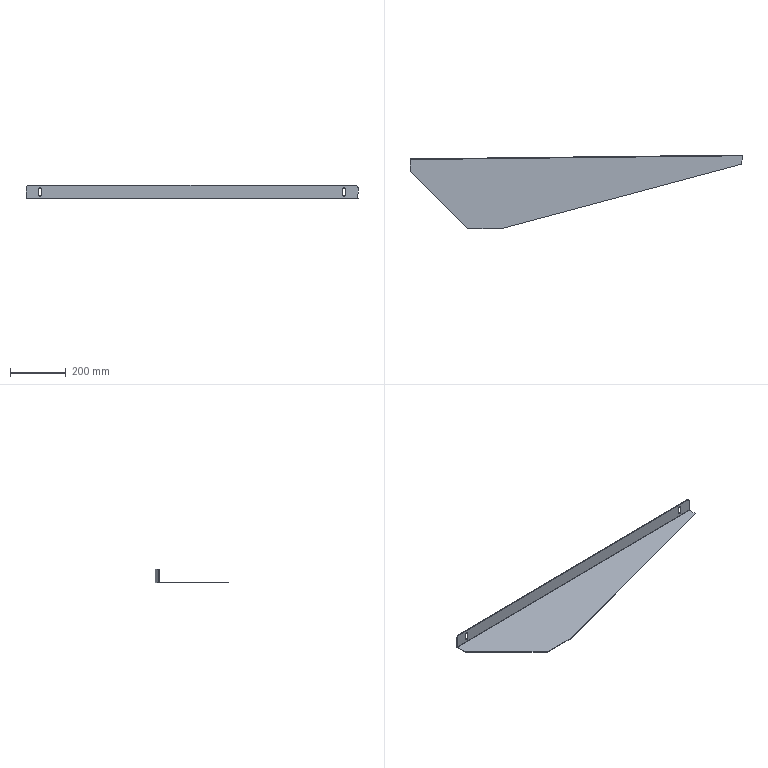Part | SolidWorks | features EdgeFlange 1, Extrusion 1, Fillet 1, FlatPattern 1, ICE 1, SheetMetal 1, SolidToSheetMetal 1 | 1 solid | 28 faces | box 1189 x 264.437 x 50 mm | volume 360864 mm3 | plane 19 | cylinder 8 | spline 1 | commonest cylinder face diameters 10 x4 20 x2 2 x1 5 x1
STEP:
#1=CARTESIAN_POINT('',(-18.814,-1.205,1.5));
#2=VERTEX_POINT('',#1);
#3=CARTESIAN_POINT('',(-18.814,-41.882,1.5));
#4=VERTEX_POINT('',#3);
#5=CARTESIAN_POINT('',(-18.814,0.5447,1.5));
#6=DIRECTION('',(0.,-1.,0.));
#7=VECTOR('',#6,1000.);
#8=LINE('',#5,#7);
#9=EDGE_CURVE('',#2,#4,#8,.T.);
#10=ORIENTED_EDGE('',*,*,#9,.F.);
#11=CARTESIAN_POINT('',(-18.814,-1.205,0.));
#12=VERTEX_POINT('',#11);
#13=CARTESIAN_POINT('',(-18.814,-1.205,1.5));
#14=DIRECTION('',(0.,0.,-1.));
#15=VECTOR('',#14,1000.);
#16=LINE('',#13,#15);
#17=EDGE_CURVE('',#2,#12,#16,.T.);
#18=ORIENTED_EDGE('',*,*,#17,.T.);
#19=CARTESIAN_POINT('',(-18.814,-41.882,0.));
#20=VERTEX_POINT('',#19);
#21=CARTESIAN_POINT('',(-18.814,0.,0.));
#22=DIRECTION('',(0.,-1.,0.));
#23=VECTOR('',#22,1000.);
#24=LINE('',#21,#23);
#25=EDGE_CURVE('',#12,#20,#24,.T.);
#26=ORIENTED_EDGE('',*,*,#25,.T.);
#27=CARTESIAN_POINT('',(-18.814,-41.882,1.5));
#28=DIRECTION('',(0.,0.,1.));
#29=VECTOR('',#28,1000.);
#30=LINE('',#27,#29);
#31=EDGE_CURVE('',#20,#4,#30,.T.);
#32=ORIENTED_EDGE('',*,*,#31,.T.);
#33=EDGE_LOOP('',(#10,#18,#26,#32));
#34=FACE_OUTER_BOUND('',#33,.T.);
#35=CARTESIAN_POINT('',(-18.814,0.5447,1.5));
#36=DIRECTION('',(-1.,0.,0.));
#37=DIRECTION('',(0.,-1.,0.));
#38=AXIS2_PLACEMENT_3D('',#35,#36,#37);
#39=PLANE('',#38);
#40=ADVANCED_FACE('',(#34),#39,.T.);
#41=CARTESIAN_POINT('',(-18.793,-1.205,1.5));
#42=VERTEX_POINT('',#41);
#43=CARTESIAN_POINT('',(-18.802,-0.4552,1.5));
#44=VERTEX_POINT('',#43);
#45=CARTESIAN_POINT('',(-18.793,-1.205,1.5));
#46=DIRECTION('',(-0.01155,0.9999,0.));
#47=VECTOR('',#46,1000.);
#48=LINE('',#45,#47);
#49=EDGE_CURVE('',#42,#44,#48,.T.);
#50=ORIENTED_EDGE('',*,*,#49,.F.);
#51=CARTESIAN_POINT('',(-19.543,-1.214,1.5));
#52=DIRECTION('',(0.9999,0.01155,0.));
#53=VECTOR('',#52,1000.);
#54=LINE('',#51,#53);
#55=EDGE_CURVE('',#2,#42,#54,.T.);
#56=ORIENTED_EDGE('',*,*,#55,.F.);
#57=ORIENTED_EDGE('',*,*,#9,.T.);
#58=CARTESIAN_POINT('',(187.963,-248.658,1.5));
#59=VERTEX_POINT('',#58);
#60=CARTESIAN_POINT('',(-18.814,-41.882,1.5));
#61=DIRECTION('',(0.7071,-0.7071,0.));
#62=VECTOR('',#61,1000.);
#63=LINE('',#60,#62);
#64=EDGE_CURVE('',#4,#59,#63,.T.);
#65=ORIENTED_EDGE('',*,*,#64,.T.);
#66=CARTESIAN_POINT('',(304.339,-248.658,1.5));
#67=VERTEX_POINT('',#66);
#68=CARTESIAN_POINT('',(187.963,-248.658,1.5));
#69=DIRECTION('',(1.,0.,0.));
#70=VECTOR('',#69,1000.);
#71=LINE('',#68,#70);
#72=EDGE_CURVE('',#59,#67,#71,.T.);
#73=ORIENTED_EDGE('',*,*,#72,.T.);
#74=CARTESIAN_POINT('',(1169.723,-16.78,1.5));
#75=VERTEX_POINT('',#74);
#76=CARTESIAN_POINT('',(304.339,-248.658,1.5));
#77=DIRECTION('',(0.9659,0.2588,0.));
#78=VECTOR('',#77,1000.);
#79=LINE('',#76,#78);
#80=EDGE_CURVE('',#67,#75,#79,.T.);
#81=ORIENTED_EDGE('',*,*,#80,.T.);
#82=CARTESIAN_POINT('',(1169.723,13.279,1.5));
#83=VERTEX_POINT('',#82);
#84=CARTESIAN_POINT('',(1169.723,14.279,1.5));
#85=DIRECTION('',(0.,1.,0.));
#86=VECTOR('',#85,1000.);
#87=LINE('',#84,#86);
#88=EDGE_CURVE('',#75,#83,#87,.T.);
#89=ORIENTED_EDGE('',*,*,#88,.T.);
#90=CARTESIAN_POINT('',(-18.802,-0.4552,1.5));
#91=DIRECTION('',(0.9999,0.01155,0.));
#92=VECTOR('',#91,1000.);
#93=LINE('',#90,#92);
#94=EDGE_CURVE('',#44,#83,#93,.T.);
#95=ORIENTED_EDGE('',*,*,#94,.F.);
#96=EDGE_LOOP('',(#50,#56,#57,#65,#73,#81,#89,#95));
#97=FACE_OUTER_BOUND('',#96,.T.);
#98=CARTESIAN_POINT('',(0.,0.,1.5));
#99=DIRECTION('',(0.,0.,1.));
#100=DIRECTION('',(1.,0.,0.));
#101=AXIS2_PLACEMENT_3D('',#98,#99,#100);
#102=PLANE('',#101);
#103=ADVANCED_FACE('',(#97),#102,.T.);
#104=CARTESIAN_POINT('',(-18.793,-1.205,0.));
#105=VERTEX_POINT('',#104);
#106=CARTESIAN_POINT('',(0.01141,-0.9878,0.));
#107=DIRECTION('',(-0.9999,-0.01155,0.));
#108=VECTOR('',#107,1000.);
#109=LINE('',#106,#108);
#110=EDGE_CURVE('',#105,#12,#109,.T.);
#111=ORIENTED_EDGE('',*,*,#110,.F.);
#112=CARTESIAN_POINT('',(-18.802,-0.4552,0.));
#113=VERTEX_POINT('',#112);
#114=CARTESIAN_POINT('',(-18.805,-0.2173,0.));
#115=DIRECTION('',(0.01155,-0.9999,0.));
#116=VECTOR('',#115,1000.);
#117=LINE('',#114,#116);
#118=EDGE_CURVE('',#113,#105,#117,.T.);
#119=ORIENTED_EDGE('',*,*,#118,.F.);
#120=CARTESIAN_POINT('',(1169.723,13.279,0.));
#121=VERTEX_POINT('',#120);
#122=CARTESIAN_POINT('',(-18.802,-0.4552,0.));
#123=DIRECTION('',(0.9999,0.01155,0.));
#124=VECTOR('',#123,1000.);
#125=LINE('',#122,#124);
#126=EDGE_CURVE('',#113,#121,#125,.T.);
#127=ORIENTED_EDGE('',*,*,#126,.T.);
#128=CARTESIAN_POINT('',(1169.723,-16.78,0.));
#129=VERTEX_POINT('',#128);
#130=CARTESIAN_POINT('',(1169.723,0.,0.));
#131=DIRECTION('',(0.,1.,0.));
#132=VECTOR('',#131,1000.);
#133=LINE('',#130,#132);
#134=EDGE_CURVE('',#129,#121,#133,.T.);
#135=ORIENTED_EDGE('',*,*,#134,.F.);
#136=CARTESIAN_POINT('',(304.339,-248.658,0.));
#137=VERTEX_POINT('',#136);
#138=CARTESIAN_POINT('',(304.339,-248.658,0.));
#139=DIRECTION('',(0.9659,0.2588,0.));
#140=VECTOR('',#139,1000.);
#141=LINE('',#138,#140);
#142=EDGE_CURVE('',#137,#129,#141,.T.);
#143=ORIENTED_EDGE('',*,*,#142,.F.);
#144=CARTESIAN_POINT('',(187.963,-248.658,0.));
#145=VERTEX_POINT('',#144);
#146=CARTESIAN_POINT('',(0.,-248.658,0.));
#147=DIRECTION('',(1.,0.,0.));
#148=VECTOR('',#147,1000.);
#149=LINE('',#146,#148);
#150=EDGE_CURVE('',#145,#137,#149,.T.);
#151=ORIENTED_EDGE('',*,*,#150,.F.);
#152=CARTESIAN_POINT('',(-18.814,-41.882,0.));
#153=DIRECTION('',(0.7071,-0.7071,0.));
#154=VECTOR('',#153,1000.);
#155=LINE('',#152,#154);
#156=EDGE_CURVE('',#20,#145,#155,.T.);
#157=ORIENTED_EDGE('',*,*,#156,.F.);
#158=ORIENTED_EDGE('',*,*,#25,.F.);
#159=EDGE_LOOP('',(#111,#119,#127,#135,#143,#151,#157,#158));
#160=FACE_OUTER_BOUND('',#159,.T.);
#161=CARTESIAN_POINT('',(0.,0.,0.));
#162=DIRECTION('',(0.,0.,1.));
#163=DIRECTION('',(1.,0.,0.));
#164=AXIS2_PLACEMENT_3D('',#161,#162,#163);
#165=PLANE('',#164);
#166=ADVANCED_FACE('',(#160),#165,.F.);
#167=ORIENTED_EDGE('',*,*,#31,.F.);
#168=ORIENTED_EDGE('',*,*,#156,.T.);
#169=CARTESIAN_POINT('',(187.963,-248.658,1.5));
#170=DIRECTION('',(0.,0.,1.));
#171=VECTOR('',#170,1000.);
#172=LINE('',#169,#171);
#173=EDGE_CURVE('',#145,#59,#172,.T.);
#174=ORIENTED_EDGE('',*,*,#173,.T.);
#175=ORIENTED_EDGE('',*,*,#64,.F.);
#176=EDGE_LOOP('',(#167,#168,#174,#175));
#177=FACE_OUTER_BOUND('',#176,.T.);
#178=CARTESIAN_POINT('',(-18.814,-41.882,1.5));
#179=DIRECTION('',(-0.7071,-0.7071,0.));
#180=DIRECTION('',(0.7071,-0.7071,0.));
#181=AXIS2_PLACEMENT_3D('',#178,#179,#180);
#182=PLANE('',#181);
#183=ADVANCED_FACE('',(#177),#182,.T.);
#184=ORIENTED_EDGE('',*,*,#173,.F.);
#185=ORIENTED_EDGE('',*,*,#150,.T.);
#186=CARTESIAN_POINT('',(304.339,-248.658,1.5));
#187=DIRECTION('',(0.,0.,1.));
#188=VECTOR('',#187,1000.);
#189=LINE('',#186,#188);
#190=EDGE_CURVE('',#137,#67,#189,.T.);
#191=ORIENTED_EDGE('',*,*,#190,.T.);
#192=ORIENTED_EDGE('',*,*,#72,.F.);
#193=EDGE_LOOP('',(#184,#185,#191,#192));
#194=FACE_OUTER_BOUND('',#193,.T.);
#195=CARTESIAN_POINT('',(187.963,-248.658,1.5));
#196=DIRECTION('',(0.,-1.,0.));
#197=DIRECTION('',(1.,0.,0.));
#198=AXIS2_PLACEMENT_3D('',#195,#196,#197);
#199=PLANE('',#198);
#200=ADVANCED_FACE('',(#194),#199,.T.);
#201=ORIENTED_EDGE('',*,*,#190,.F.);
#202=ORIENTED_EDGE('',*,*,#142,.T.);
#203=CARTESIAN_POINT('',(1169.723,-16.78,1.5));
#204=DIRECTION('',(0.,0.,1.));
#205=VECTOR('',#204,1000.);
#206=LINE('',#203,#205);
#207=EDGE_CURVE('',#129,#75,#206,.T.);
#208=ORIENTED_EDGE('',*,*,#207,.T.);
#209=ORIENTED_EDGE('',*,*,#80,.F.);
#210=EDGE_LOOP('',(#201,#202,#208,#209));
#211=FACE_OUTER_BOUND('',#210,.T.);
#212=CARTESIAN_POINT('',(304.339,-248.658,1.5));
#213=DIRECTION('',(0.2588,-0.9659,0.));
#214=DIRECTION('',(0.9659,0.2588,0.));
#215=AXIS2_PLACEMENT_3D('',#212,#213,#214);
#216=PLANE('',#215);
#217=ADVANCED_FACE('',(#211),#216,.T.);
#218=CARTESIAN_POINT('',(1169.723,13.279,1.5));
#219=DIRECTION('',(0.,0.,-1.));
#220=VECTOR('',#219,1000.);
#221=LINE('',#218,#220);
#222=EDGE_CURVE('',#83,#121,#221,.T.);
#223=ORIENTED_EDGE('',*,*,#222,.F.);
#224=ORIENTED_EDGE('',*,*,#88,.F.);
#225=ORIENTED_EDGE('',*,*,#207,.F.);
#226=ORIENTED_EDGE('',*,*,#134,.T.);
#227=EDGE_LOOP('',(#223,#224,#225,#226));
#228=FACE_OUTER_BOUND('',#227,.T.);
#229=CARTESIAN_POINT('',(1169.723,14.279,1.5));
#230=DIRECTION('',(1.,0.,0.));
#231=DIRECTION('',(0.,1.,0.));
#232=AXIS2_PLACEMENT_3D('',#229,#230,#231);
#233=PLANE('',#232);
#234=ADVANCED_FACE('',(#228),#233,.T.);
#235=CARTESIAN_POINT('',(-18.802,-0.4552,1.5));
#236=DIRECTION('',(0.,0.,-1.));
#237=VECTOR('',#236,1000.);
#238=LINE('',#235,#237);
#239=EDGE_CURVE('',#44,#113,#238,.T.);
#240=ORIENTED_EDGE('',*,*,#239,.T.);
#241=ORIENTED_EDGE('',*,*,#118,.T.);
#242=CARTESIAN_POINT('',(-18.793,-1.205,1.5));
#243=DIRECTION('',(0.,0.,-1.));
#244=VECTOR('',#243,1000.);
#245=LINE('',#242,#244);
#246=EDGE_CURVE('',#42,#105,#245,.T.);
#247=ORIENTED_EDGE('',*,*,#246,.F.);
#248=ORIENTED_EDGE('',*,*,#49,.T.);
#249=EDGE_LOOP('',(#240,#241,#247,#248));
#250=FACE_OUTER_BOUND('',#249,.T.);
#251=CARTESIAN_POINT('',(-18.793,-1.205,1.5));
#252=DIRECTION('',(-0.9999,-0.01155,0.));
#253=DIRECTION('',(0.01155,-0.9999,0.));
#254=AXIS2_PLACEMENT_3D('',#251,#252,#253);
#255=PLANE('',#254);
#256=ADVANCED_FACE('',(#250),#255,.T.);
#257=ORIENTED_EDGE('',*,*,#17,.F.);
#258=ORIENTED_EDGE('',*,*,#55,.T.);
#259=ORIENTED_EDGE('',*,*,#246,.T.);
#260=ORIENTED_EDGE('',*,*,#110,.T.);
#261=EDGE_LOOP('',(#257,#258,#259,#260));
#262=FACE_OUTER_BOUND('',#261,.T.);
#263=CARTESIAN_POINT('',(-19.543,-1.214,1.5));
#264=DIRECTION('',(-0.01155,0.9999,0.));
#265=DIRECTION('',(-0.9999,-0.01155,0.));
#266=AXIS2_PLACEMENT_3D('',#263,#264,#265);
#267=PLANE('',#266);
#268=ADVANCED_FACE('',(#262),#267,.T.);
#269=CARTESIAN_POINT('',(1169.723,14.279,2.5));
#270=VERTEX_POINT('',#269);
#271=CARTESIAN_POINT('',(1169.705,15.779,2.5));
#272=VERTEX_POINT('',#271);
#273=CARTESIAN_POINT('',(1169.723,14.279,2.5));
#274=DIRECTION('',(-0.01155,0.9999,0.));
#275=VECTOR('',#274,1000.);
#276=LINE('',#273,#275);
#277=EDGE_CURVE('',#270,#272,#276,.T.);
#278=ORIENTED_EDGE('',*,*,#277,.F.);
#279=CARTESIAN_POINT('',(1169.723,13.279,1.5));
#280=CARTESIAN_POINT('',(1169.722,13.541,1.5));
#281=CARTESIAN_POINT('',(1169.721,13.801,1.608));
#282=CARTESIAN_POINT('',(1169.72,14.171,1.978));
#283=CARTESIAN_POINT('',(1169.721,14.279,2.238));
#284=CARTESIAN_POINT('',(1169.723,14.279,2.5));
#285=B_SPLINE_CURVE_WITH_KNOTS('',3,(#279,#280,#281,#282,#283,#284),.UNSPECIFIED.,.F.,.F.,(4,2,4),(0.,0.5,1.),.UNSPECIFIED.);
#286=EDGE_CURVE('',#83,#270,#285,.T.);
#287=ORIENTED_EDGE('',*,*,#286,.F.);
#288=ORIENTED_EDGE('',*,*,#222,.T.);
#289=CARTESIAN_POINT('',(1169.723,13.279,0.));
#290=CARTESIAN_POINT('',(1169.72,13.606,0.));
#291=CARTESIAN_POINT('',(1169.717,13.933,0.06507));
#292=CARTESIAN_POINT('',(1169.712,14.538,0.3155));
#293=CARTESIAN_POINT('',(1169.71,14.815,0.5008));
#294=CARTESIAN_POINT('',(1169.706,15.278,0.9636));
#295=CARTESIAN_POINT('',(1169.705,15.463,1.241));
#296=CARTESIAN_POINT('',(1169.704,15.714,1.846));
#297=CARTESIAN_POINT('',(1169.704,15.779,2.173));
#298=CARTESIAN_POINT('',(1169.705,15.779,2.5));
#299=B_SPLINE_CURVE_WITH_KNOTS('',3,(#289,#290,#291,#292,#293,#294,#295,#296,#297,#298),.UNSPECIFIED.,.F.,.F.,(4,2,2,2,4),(0.,0.25,0.5,0.75,1.),.UNSPECIFIED.);
#300=EDGE_CURVE('',#121,#272,#299,.T.);
#301=ORIENTED_EDGE('',*,*,#300,.T.);
#302=EDGE_LOOP('',(#278,#287,#288,#301));
#303=FACE_OUTER_BOUND('',#302,.T.);
#304=CARTESIAN_POINT('',(1169.723,13.279,-0.015));
#305=CARTESIAN_POINT('',(1169.72,13.608,-0.015));
#306=CARTESIAN_POINT('',(1169.717,13.937,0.05046));
#307=CARTESIAN_POINT('',(1169.712,14.545,0.3024));
#308=CARTESIAN_POINT('',(1169.71,14.824,0.4888));
#309=CARTESIAN_POINT('',(1169.706,15.29,0.9544));
#310=CARTESIAN_POINT('',(1169.705,15.476,1.233));
#311=CARTESIAN_POINT('',(1169.704,15.728,1.842));
#312=CARTESIAN_POINT('',(1169.704,15.794,2.171));
#313=CARTESIAN_POINT('',(1169.705,15.794,2.5));
#314=CARTESIAN_POINT('',(1169.723,13.279,0.));
#315=CARTESIAN_POINT('',(1169.72,13.606,0.));
#316=CARTESIAN_POINT('',(1169.717,13.933,0.06507));
#317=CARTESIAN_POINT('',(1169.712,14.538,0.3155));
#318=CARTESIAN_POINT('',(1169.71,14.815,0.5008));
#319=CARTESIAN_POINT('',(1169.706,15.278,0.9636));
#320=CARTESIAN_POINT('',(1169.705,15.463,1.241));
#321=CARTESIAN_POINT('',(1169.704,15.714,1.846));
#322=CARTESIAN_POINT('',(1169.704,15.779,2.173));
#323=CARTESIAN_POINT('',(1169.705,15.779,2.5));
#324=CARTESIAN_POINT('',(1169.723,13.279,1.5));
#325=CARTESIAN_POINT('',(1169.722,13.41,1.5));
#326=CARTESIAN_POINT('',(1169.722,13.54,1.526));
#327=CARTESIAN_POINT('',(1169.721,13.782,1.626));
#328=CARTESIAN_POINT('',(1169.72,13.893,1.7));
#329=CARTESIAN_POINT('',(1169.72,14.078,1.885));
#330=CARTESIAN_POINT('',(1169.72,14.153,1.996));
#331=CARTESIAN_POINT('',(1169.721,14.253,2.238));
#332=CARTESIAN_POINT('',(1169.722,14.279,2.369));
#333=CARTESIAN_POINT('',(1169.723,14.279,2.5));
#334=CARTESIAN_POINT('',(1169.723,13.279,1.515));
#335=CARTESIAN_POINT('',(1169.722,13.408,1.515));
#336=CARTESIAN_POINT('',(1169.722,13.537,1.541));
#337=CARTESIAN_POINT('',(1169.721,13.775,1.639));
#338=CARTESIAN_POINT('',(1169.721,13.884,1.712));
#339=CARTESIAN_POINT('',(1169.72,14.066,1.895));
#340=CARTESIAN_POINT('',(1169.72,14.139,2.004));
#341=CARTESIAN_POINT('',(1169.721,14.238,2.242));
#342=CARTESIAN_POINT('',(1169.722,14.264,2.371));
#343=CARTESIAN_POINT('',(1169.723,14.264,2.5));
#344=B_SPLINE_SURFACE_WITH_KNOTS('',1,3,((#304,#305,#306,#307,#308,#309,#310,#311,#312,#313),(#314,#315,#316,#317,#318,#319,#320,#321,#322,#323),(#324,#325,#326,#327,#328,#329,#330,#331,#332,#333),(#334,#335,#336,#337,#338,#339,#340,#341,#342,#343)),.UNSPECIFIED.,.F.,.F.,.F.,(2,1,1,2),(4,2,2,2,4),(-0.01,0.,1.,1.01),(0.,0.25,0.5,0.75,1.),.UNSPECIFIED.);
#345=ADVANCED_FACE('',(#303),#344,.F.);
#346=CARTESIAN_POINT('',(-18.814,0.5447,2.5));
#347=VERTEX_POINT('',#346);
#348=CARTESIAN_POINT('',(-18.802,-0.4552,2.5));
#349=DIRECTION('',(-0.9999,-0.01155,0.));
#350=DIRECTION('',(0.01155,-0.9999,0.));
#351=AXIS2_PLACEMENT_3D('',#348,#349,#350);
#352=CIRCLE('',#351,1.);
#353=EDGE_CURVE('',#347,#44,#352,.T.);
#354=ORIENTED_EDGE('',*,*,#353,.F.);
#355=CARTESIAN_POINT('',(-18.831,2.045,2.5));
#356=VERTEX_POINT('',#355);
#357=CARTESIAN_POINT('',(-18.814,0.5447,2.5));
#358=DIRECTION('',(-0.01155,0.9999,0.));
#359=VECTOR('',#358,1000.);
#360=LINE('',#357,#359);
#361=EDGE_CURVE('',#347,#356,#360,.T.);
#362=ORIENTED_EDGE('',*,*,#361,.T.);
#363=CARTESIAN_POINT('',(-18.802,-0.4552,2.5));
#364=DIRECTION('',(-0.9999,-0.01155,0.));
#365=DIRECTION('',(0.01155,-0.9999,0.));
#366=AXIS2_PLACEMENT_3D('',#363,#364,#365);
#367=CIRCLE('',#366,2.5);
#368=EDGE_CURVE('',#356,#113,#367,.T.);
#369=ORIENTED_EDGE('',*,*,#368,.T.);
#370=ORIENTED_EDGE('',*,*,#239,.F.);
#371=EDGE_LOOP('',(#354,#362,#369,#370));
#372=FACE_OUTER_BOUND('',#371,.T.);
#373=CARTESIAN_POINT('',(-18.802,-0.4552,2.5));
#374=DIRECTION('',(0.9999,0.01155,0.));
#375=DIRECTION('',(-0.01155,0.9999,0.));
#376=AXIS2_PLACEMENT_3D('',#373,#374,#375);
#377=PLANE('',#376);
#378=ADVANCED_FACE('',(#372),#377,.F.);
#379=ORIENTED_EDGE('',*,*,#126,.F.);
#380=ORIENTED_EDGE('',*,*,#368,.F.);
#381=CARTESIAN_POINT('',(-0.02614,2.262,2.5));
#382=DIRECTION('',(0.9999,0.01155,0.));
#383=VECTOR('',#382,1000.);
#384=LINE('',#381,#383);
#385=EDGE_CURVE('',#356,#272,#384,.T.);
#386=ORIENTED_EDGE('',*,*,#385,.T.);
#387=ORIENTED_EDGE('',*,*,#300,.F.);
#388=EDGE_LOOP('',(#379,#380,#386,#387));
#389=FACE_OUTER_BOUND('',#388,.T.);
#390=CARTESIAN_POINT('',(-18.802,-0.4552,2.5));
#391=DIRECTION('',(-0.9999,-0.01155,0.));
#392=DIRECTION('',(-0.01155,0.9999,0.));
#393=AXIS2_PLACEMENT_3D('',#390,#391,#392);
#394=CYLINDRICAL_SURFACE('',#393,2.5);
#395=ADVANCED_FACE('',(#389),#394,.T.);
#396=ORIENTED_EDGE('',*,*,#94,.T.);
#397=ORIENTED_EDGE('',*,*,#286,.T.);
#398=CARTESIAN_POINT('',(1169.723,14.279,2.5));
#399=DIRECTION('',(-0.9999,-0.01155,0.));
#400=VECTOR('',#399,1000.);
#401=LINE('',#398,#400);
#402=EDGE_CURVE('',#270,#347,#401,.T.);
#403=ORIENTED_EDGE('',*,*,#402,.T.);
#404=ORIENTED_EDGE('',*,*,#353,.T.);
#405=EDGE_LOOP('',(#396,#397,#403,#404));
#406=FACE_OUTER_BOUND('',#405,.T.);
#407=CARTESIAN_POINT('',(-18.802,-0.4552,2.5));
#408=DIRECTION('',(-0.9999,-0.01155,0.));
#409=DIRECTION('',(-0.01155,0.9999,0.));
#410=AXIS2_PLACEMENT_3D('',#407,#408,#409);
#411=CYLINDRICAL_SURFACE('',#410,1.);
#412=ADVANCED_FACE('',(#406),#411,.F.);
#413=CARTESIAN_POINT('',(1169.705,15.779,40.));
#414=VERTEX_POINT('',#413);
#415=CARTESIAN_POINT('',(1169.705,15.779,1.5));
#416=DIRECTION('',(0.,0.,1.));
#417=VECTOR('',#416,1000.);
#418=LINE('',#415,#417);
#419=EDGE_CURVE('',#272,#414,#418,.T.);
#420=ORIENTED_EDGE('',*,*,#419,.T.);
#421=CARTESIAN_POINT('',(1169.723,14.279,40.));
#422=VERTEX_POINT('',#421);
#423=CARTESIAN_POINT('',(1169.705,15.779,40.));
#424=DIRECTION('',(0.01155,-0.9999,0.));
#425=VECTOR('',#424,1000.);
#426=LINE('',#423,#425);
#427=EDGE_CURVE('',#414,#422,#426,.T.);
#428=ORIENTED_EDGE('',*,*,#427,.T.);
#429=CARTESIAN_POINT('',(1169.723,14.279,1.5));
#430=DIRECTION('',(0.,0.,1.));
#431=VECTOR('',#430,1000.);
#432=LINE('',#429,#431);
#433=EDGE_CURVE('',#270,#422,#432,.T.);
#434=ORIENTED_EDGE('',*,*,#433,.F.);
#435=ORIENTED_EDGE('',*,*,#277,.T.);
#436=EDGE_LOOP('',(#420,#428,#434,#435));
#437=FACE_OUTER_BOUND('',#436,.T.);
#438=CARTESIAN_POINT('',(1169.705,15.779,1.5));
#439=DIRECTION('',(0.9999,0.01155,0.));
#440=DIRECTION('',(-0.01155,0.9999,0.));
#441=AXIS2_PLACEMENT_3D('',#438,#439,#440);
#442=PLANE('',#441);
#443=ADVANCED_FACE('',(#437),#442,.T.);
#444=CARTESIAN_POINT('',(-18.814,0.5447,40.));
#445=VERTEX_POINT('',#444);
#446=CARTESIAN_POINT('',(-18.814,0.5447,50.));
#447=DIRECTION('',(0.,0.,-1.));
#448=VECTOR('',#447,1000.);
#449=LINE('',#446,#448);
#450=EDGE_CURVE('',#445,#347,#449,.T.);
#451=ORIENTED_EDGE('',*,*,#450,.F.);
#452=CARTESIAN_POINT('',(-18.831,2.045,40.));
#453=VERTEX_POINT('',#452);
#454=CARTESIAN_POINT('',(-18.831,2.045,40.));
#455=DIRECTION('',(-0.01155,0.9999,0.));
#456=VECTOR('',#455,1000.);
#457=LINE('',#454,#456);
#458=EDGE_CURVE('',#445,#453,#457,.T.);
#459=ORIENTED_EDGE('',*,*,#458,.T.);
#460=CARTESIAN_POINT('',(-18.831,2.045,50.));
#461=DIRECTION('',(0.,0.,-1.));
#462=VECTOR('',#461,1000.);
#463=LINE('',#460,#462);
#464=EDGE_CURVE('',#453,#356,#463,.T.);
#465=ORIENTED_EDGE('',*,*,#464,.T.);
#466=ORIENTED_EDGE('',*,*,#361,.F.);
#467=EDGE_LOOP('',(#451,#459,#465,#466));
#468=FACE_OUTER_BOUND('',#467,.T.);
#469=CARTESIAN_POINT('',(-18.831,2.045,50.));
#470=DIRECTION('',(-0.9999,-0.01155,0.));
#471=DIRECTION('',(0.01155,-0.9999,0.));
#472=AXIS2_PLACEMENT_3D('',#469,#470,#471);
#473=PLANE('',#472);
#474=ADVANCED_FACE('',(#468),#473,.T.);
#475=CARTESIAN_POINT('',(26.166,2.565,15.));
#476=VERTEX_POINT('',#475);
#477=CARTESIAN_POINT('',(26.166,2.565,35.));
#478=VERTEX_POINT('',#477);
#479=CARTESIAN_POINT('',(26.166,2.565,15.));
#480=DIRECTION('',(0.,0.,1.));
#481=VECTOR('',#480,1000.);
#482=LINE('',#479,#481);
#483=EDGE_CURVE('',#476,#478,#482,.T.);
#484=ORIENTED_EDGE('',*,*,#483,.F.);
#485=CARTESIAN_POINT('',(36.165,2.68,15.));
#486=VERTEX_POINT('',#485);
#487=CARTESIAN_POINT('',(31.166,2.622,15.));
#488=DIRECTION('',(-0.01155,0.9999,0.));
#489=DIRECTION('',(-0.9999,-0.01155,0.));
#490=AXIS2_PLACEMENT_3D('',#487,#488,#489);
#491=CIRCLE('',#490,5.);
#492=EDGE_CURVE('',#486,#476,#491,.T.);
#493=ORIENTED_EDGE('',*,*,#492,.F.);
#494=CARTESIAN_POINT('',(36.165,2.68,35.));
#495=VERTEX_POINT('',#494);
#496=CARTESIAN_POINT('',(36.165,2.68,15.));
#497=DIRECTION('',(0.,0.,-1.));
#498=VECTOR('',#497,1000.);
#499=LINE('',#496,#498);
#500=EDGE_CURVE('',#495,#486,#499,.T.);
#501=ORIENTED_EDGE('',*,*,#500,.F.);
#502=CARTESIAN_POINT('',(31.166,2.622,35.));
#503=DIRECTION('',(-0.01155,0.9999,0.));
#504=DIRECTION('',(-0.9999,-0.01155,0.));
#505=AXIS2_PLACEMENT_3D('',#502,#503,#504);
#506=CIRCLE('',#505,5.);
#507=EDGE_CURVE('',#478,#495,#506,.T.);
#508=ORIENTED_EDGE('',*,*,#507,.F.);
#509=EDGE_LOOP('',(#484,#493,#501,#508));
#510=FACE_BOUND('',#509,.T.);
#511=CARTESIAN_POINT('',(1114.709,15.143,15.));
#512=VERTEX_POINT('',#511);
#513=CARTESIAN_POINT('',(1114.709,15.143,35.));
#514=VERTEX_POINT('',#513);
#515=CARTESIAN_POINT('',(1114.709,15.143,15.));
#516=DIRECTION('',(0.,0.,1.));
#517=VECTOR('',#516,1000.);
#518=LINE('',#515,#517);
#519=EDGE_CURVE('',#512,#514,#518,.T.);
#520=ORIENTED_EDGE('',*,*,#519,.F.);
#521=CARTESIAN_POINT('',(1124.708,15.259,15.));
#522=VERTEX_POINT('',#521);
#523=CARTESIAN_POINT('',(1119.709,15.201,15.));
#524=DIRECTION('',(-0.01155,0.9999,0.));
#525=DIRECTION('',(-0.9999,-0.01155,0.));
#526=AXIS2_PLACEMENT_3D('',#523,#524,#525);
#527=CIRCLE('',#526,5.);
#528=EDGE_CURVE('',#522,#512,#527,.T.);
#529=ORIENTED_EDGE('',*,*,#528,.F.);
#530=CARTESIAN_POINT('',(1124.708,15.259,35.));
#531=VERTEX_POINT('',#530);
#532=CARTESIAN_POINT('',(1124.708,15.259,15.));
#533=DIRECTION('',(0.,0.,-1.));
#534=VECTOR('',#533,1000.);
#535=LINE('',#532,#534);
#536=EDGE_CURVE('',#531,#522,#535,.T.);
#537=ORIENTED_EDGE('',*,*,#536,.F.);
#538=CARTESIAN_POINT('',(1119.709,15.201,35.));
#539=DIRECTION('',(-0.01155,0.9999,0.));
#540=DIRECTION('',(-0.9999,-0.01155,0.));
#541=AXIS2_PLACEMENT_3D('',#538,#539,#540);
#542=CIRCLE('',#541,5.);
#543=EDGE_CURVE('',#514,#531,#542,.T.);
#544=ORIENTED_EDGE('',*,*,#543,.F.);
#545=EDGE_LOOP('',(#520,#529,#537,#544));
#546=FACE_BOUND('',#545,.T.);
#547=CARTESIAN_POINT('',(1159.706,15.663,50.));
#548=VERTEX_POINT('',#547);
#549=CARTESIAN_POINT('',(-8.832,2.16,50.));
#550=VERTEX_POINT('',#549);
#551=CARTESIAN_POINT('',(1169.705,15.779,50.));
#552=DIRECTION('',(-0.9999,-0.01155,0.));
#553=VECTOR('',#552,1000.);
#554=LINE('',#551,#553);
#555=EDGE_CURVE('',#548,#550,#554,.T.);
#556=ORIENTED_EDGE('',*,*,#555,.F.);
#557=CARTESIAN_POINT('',(1159.706,15.663,40.));
#558=DIRECTION('',(-0.01155,0.9999,0.));
#559=DIRECTION('',(0.9999,0.01155,0.));
#560=AXIS2_PLACEMENT_3D('',#557,#558,#559);
#561=CIRCLE('',#560,10.);
#562=EDGE_CURVE('',#548,#414,#561,.T.);
#563=ORIENTED_EDGE('',*,*,#562,.T.);
#564=ORIENTED_EDGE('',*,*,#419,.F.);
#565=ORIENTED_EDGE('',*,*,#385,.F.);
#566=ORIENTED_EDGE('',*,*,#464,.F.);
#567=CARTESIAN_POINT('',(-8.832,2.16,40.));
#568=DIRECTION('',(-0.01155,0.9999,0.));
#569=DIRECTION('',(0.9999,0.01155,0.));
#570=AXIS2_PLACEMENT_3D('',#567,#568,#569);
#571=CIRCLE('',#570,10.);
#572=EDGE_CURVE('',#453,#550,#571,.T.);
#573=ORIENTED_EDGE('',*,*,#572,.T.);
#574=EDGE_LOOP('',(#556,#563,#564,#565,#566,#573));
#575=FACE_OUTER_BOUND('',#574,.T.);
#576=CARTESIAN_POINT('',(-0.02614,2.262,0.));
#577=DIRECTION('',(0.01155,-0.9999,0.));
#578=DIRECTION('',(0.9999,0.01155,0.));
#579=AXIS2_PLACEMENT_3D('',#576,#577,#578);
#580=PLANE('',#579);
#581=ADVANCED_FACE('',(#510,#546,#575),#580,.F.);
#582=CARTESIAN_POINT('',(26.183,1.065,15.));
#583=VERTEX_POINT('',#582);
#584=CARTESIAN_POINT('',(36.183,1.18,15.));
#585=VERTEX_POINT('',#584);
#586=CARTESIAN_POINT('',(31.183,1.122,15.));
#587=DIRECTION('',(0.01155,-0.9999,0.));
#588=DIRECTION('',(0.9999,0.01155,0.));
#589=AXIS2_PLACEMENT_3D('',#586,#587,#588);
#590=CIRCLE('',#589,5.);
#591=EDGE_CURVE('',#583,#585,#590,.T.);
#592=ORIENTED_EDGE('',*,*,#591,.F.);
#593=CARTESIAN_POINT('',(26.183,1.065,35.));
#594=VERTEX_POINT('',#593);
#595=CARTESIAN_POINT('',(26.183,1.065,0.));
#596=DIRECTION('',(0.,0.,-1.));
#597=VECTOR('',#596,1000.);
#598=LINE('',#595,#597);
#599=EDGE_CURVE('',#594,#583,#598,.T.);
#600=ORIENTED_EDGE('',*,*,#599,.F.);
#601=CARTESIAN_POINT('',(36.183,1.18,35.));
#602=VERTEX_POINT('',#601);
#603=CARTESIAN_POINT('',(31.183,1.122,35.));
#604=DIRECTION('',(0.01155,-0.9999,0.));
#605=DIRECTION('',(0.9999,0.01155,0.));
#606=AXIS2_PLACEMENT_3D('',#603,#604,#605);
#607=CIRCLE('',#606,5.);
#608=EDGE_CURVE('',#602,#594,#607,.T.);
#609=ORIENTED_EDGE('',*,*,#608,.F.);
#610=CARTESIAN_POINT('',(36.183,1.18,0.));
#611=DIRECTION('',(0.,0.,1.));
#612=VECTOR('',#611,1000.);
#613=LINE('',#610,#612);
#614=EDGE_CURVE('',#585,#602,#613,.T.);
#615=ORIENTED_EDGE('',*,*,#614,.F.);
#616=EDGE_LOOP('',(#592,#600,#609,#615));
#617=FACE_BOUND('',#616,.T.);
#618=CARTESIAN_POINT('',(1114.726,13.643,15.));
#619=VERTEX_POINT('',#618);
#620=CARTESIAN_POINT('',(1124.726,13.759,15.));
#621=VERTEX_POINT('',#620);
#622=CARTESIAN_POINT('',(1119.726,13.701,15.));
#623=DIRECTION('',(0.01155,-0.9999,0.));
#624=DIRECTION('',(0.9999,0.01155,0.));
#625=AXIS2_PLACEMENT_3D('',#622,#623,#624);
#626=CIRCLE('',#625,5.);
#627=EDGE_CURVE('',#619,#621,#626,.T.);
#628=ORIENTED_EDGE('',*,*,#627,.F.);
#629=CARTESIAN_POINT('',(1114.726,13.643,35.));
#630=VERTEX_POINT('',#629);
#631=CARTESIAN_POINT('',(1114.726,13.643,0.));
#632=DIRECTION('',(0.,0.,-1.));
#633=VECTOR('',#632,1000.);
#634=LINE('',#631,#633);
#635=EDGE_CURVE('',#630,#619,#634,.T.);
#636=ORIENTED_EDGE('',*,*,#635,.F.);
#637=CARTESIAN_POINT('',(1124.726,13.759,35.));
#638=VERTEX_POINT('',#637);
#639=CARTESIAN_POINT('',(1119.726,13.701,35.));
#640=DIRECTION('',(0.01155,-0.9999,0.));
#641=DIRECTION('',(0.9999,0.01155,0.));
#642=AXIS2_PLACEMENT_3D('',#639,#640,#641);
#643=CIRCLE('',#642,5.);
#644=EDGE_CURVE('',#638,#630,#643,.T.);
#645=ORIENTED_EDGE('',*,*,#644,.F.);
#646=CARTESIAN_POINT('',(1124.726,13.759,0.));
#647=DIRECTION('',(0.,0.,1.));
#648=VECTOR('',#647,1000.);
#649=LINE('',#646,#648);
#650=EDGE_CURVE('',#621,#638,#649,.T.);
#651=ORIENTED_EDGE('',*,*,#650,.F.);
#652=EDGE_LOOP('',(#628,#636,#645,#651));
#653=FACE_BOUND('',#652,.T.);
#654=ORIENTED_EDGE('',*,*,#433,.T.);
#655=CARTESIAN_POINT('',(1159.723,14.163,50.));
#656=VERTEX_POINT('',#655);
#657=CARTESIAN_POINT('',(1159.723,14.163,40.));
#658=DIRECTION('',(0.01155,-0.9999,0.));
#659=DIRECTION('',(0.9999,0.01155,0.));
#660=AXIS2_PLACEMENT_3D('',#657,#658,#659);
#661=CIRCLE('',#660,10.);
#662=EDGE_CURVE('',#422,#656,#661,.T.);
#663=ORIENTED_EDGE('',*,*,#662,.T.);
#664=CARTESIAN_POINT('',(-8.814,0.6603,50.));
#665=VERTEX_POINT('',#664);
#666=CARTESIAN_POINT('',(1169.723,14.279,50.));
#667=DIRECTION('',(-0.9999,-0.01155,0.));
#668=VECTOR('',#667,1000.);
#669=LINE('',#666,#668);
#670=EDGE_CURVE('',#656,#665,#669,.T.);
#671=ORIENTED_EDGE('',*,*,#670,.T.);
#672=CARTESIAN_POINT('',(-8.814,0.6603,40.));
#673=DIRECTION('',(0.01155,-0.9999,0.));
#674=DIRECTION('',(0.9999,0.01155,0.));
#675=AXIS2_PLACEMENT_3D('',#672,#673,#674);
#676=CIRCLE('',#675,10.);
#677=EDGE_CURVE('',#665,#445,#676,.T.);
#678=ORIENTED_EDGE('',*,*,#677,.T.);
#679=ORIENTED_EDGE('',*,*,#450,.T.);
#680=ORIENTED_EDGE('',*,*,#402,.F.);
#681=EDGE_LOOP('',(#654,#663,#671,#678,#679,#680));
#682=FACE_OUTER_BOUND('',#681,.T.);
#683=CARTESIAN_POINT('',(-0.008806,0.762,0.));
#684=DIRECTION('',(0.01155,-0.9999,0.));
#685=DIRECTION('',(0.9999,0.01155,0.));
#686=AXIS2_PLACEMENT_3D('',#683,#684,#685);
#687=PLANE('',#686);
#688=ADVANCED_FACE('',(#617,#653,#682),#687,.T.);
#689=ORIENTED_EDGE('',*,*,#670,.F.);
#690=CARTESIAN_POINT('',(1159.706,15.663,50.));
#691=DIRECTION('',(-0.01155,0.9999,0.));
#692=VECTOR('',#691,1000.);
#693=LINE('',#690,#692);
#694=EDGE_CURVE('',#656,#548,#693,.T.);
#695=ORIENTED_EDGE('',*,*,#694,.T.);
#696=ORIENTED_EDGE('',*,*,#555,.T.);
#697=CARTESIAN_POINT('',(-8.832,2.16,50.));
#698=DIRECTION('',(0.01155,-0.9999,0.));
#699=VECTOR('',#698,1000.);
#700=LINE('',#697,#699);
#701=EDGE_CURVE('',#550,#665,#700,.T.);
#702=ORIENTED_EDGE('',*,*,#701,.T.);
#703=EDGE_LOOP('',(#689,#695,#696,#702));
#704=FACE_OUTER_BOUND('',#703,.T.);
#705=CARTESIAN_POINT('',(1169.705,15.779,50.));
#706=DIRECTION('',(0.,0.,1.));
#707=DIRECTION('',(0.,-1.,0.));
#708=AXIS2_PLACEMENT_3D('',#705,#706,#707);
#709=PLANE('',#708);
#710=ADVANCED_FACE('',(#704),#709,.T.);
#711=ORIENTED_EDGE('',*,*,#627,.T.);
#712=CARTESIAN_POINT('',(1124.824,5.259,15.));
#713=DIRECTION('',(-0.01155,0.9999,0.));
#714=VECTOR('',#713,1000.);
#715=LINE('',#712,#714);
#716=EDGE_CURVE('',#621,#522,#715,.T.);
#717=ORIENTED_EDGE('',*,*,#716,.T.);
#718=ORIENTED_EDGE('',*,*,#528,.T.);
#719=CARTESIAN_POINT('',(1114.825,5.144,15.));
#720=DIRECTION('',(-0.01155,0.9999,0.));
#721=VECTOR('',#720,1000.);
#722=LINE('',#719,#721);
#723=EDGE_CURVE('',#619,#512,#722,.T.);
#724=ORIENTED_EDGE('',*,*,#723,.F.);
#725=EDGE_LOOP('',(#711,#717,#718,#724));
#726=FACE_OUTER_BOUND('',#725,.T.);
#727=CARTESIAN_POINT('',(1119.824,5.202,15.));
#728=DIRECTION('',(-0.01155,0.9999,0.));
#729=DIRECTION('',(-0.9999,-0.01155,0.));
#730=AXIS2_PLACEMENT_3D('',#727,#728,#729);
#731=CYLINDRICAL_SURFACE('',#730,5.);
#732=ADVANCED_FACE('',(#726),#731,.F.);
#733=ORIENTED_EDGE('',*,*,#650,.T.);
#734=CARTESIAN_POINT('',(1124.824,5.259,35.));
#735=DIRECTION('',(-0.01155,0.9999,0.));
#736=VECTOR('',#735,1000.);
#737=LINE('',#734,#736);
#738=EDGE_CURVE('',#638,#531,#737,.T.);
#739=ORIENTED_EDGE('',*,*,#738,.T.);
#740=ORIENTED_EDGE('',*,*,#536,.T.);
#741=ORIENTED_EDGE('',*,*,#716,.F.);
#742=EDGE_LOOP('',(#733,#739,#740,#741));
#743=FACE_OUTER_BOUND('',#742,.T.);
#744=CARTESIAN_POINT('',(1124.824,5.259,15.));
#745=DIRECTION('',(0.9999,0.01155,0.));
#746=DIRECTION('',(-0.01155,0.9999,0.));
#747=AXIS2_PLACEMENT_3D('',#744,#745,#746);
#748=PLANE('',#747);
#749=ADVANCED_FACE('',(#743),#748,.F.);
#750=ORIENTED_EDGE('',*,*,#644,.T.);
#751=CARTESIAN_POINT('',(1114.825,5.144,35.));
#752=DIRECTION('',(-0.01155,0.9999,0.));
#753=VECTOR('',#752,1000.);
#754=LINE('',#751,#753);
#755=EDGE_CURVE('',#630,#514,#754,.T.);
#756=ORIENTED_EDGE('',*,*,#755,.T.);
#757=ORIENTED_EDGE('',*,*,#543,.T.);
#758=ORIENTED_EDGE('',*,*,#738,.F.);
#759=EDGE_LOOP('',(#750,#756,#757,#758));
#760=FACE_OUTER_BOUND('',#759,.T.);
#761=CARTESIAN_POINT('',(1119.824,5.202,35.));
#762=DIRECTION('',(-0.01155,0.9999,0.));
#763=DIRECTION('',(-0.9999,-0.01155,0.));
#764=AXIS2_PLACEMENT_3D('',#761,#762,#763);
#765=CYLINDRICAL_SURFACE('',#764,5.);
#766=ADVANCED_FACE('',(#760),#765,.F.);
#767=ORIENTED_EDGE('',*,*,#635,.T.);
#768=ORIENTED_EDGE('',*,*,#723,.T.);
#769=ORIENTED_EDGE('',*,*,#519,.T.);
#770=ORIENTED_EDGE('',*,*,#755,.F.);
#771=EDGE_LOOP('',(#767,#768,#769,#770));
#772=FACE_OUTER_BOUND('',#771,.T.);
#773=CARTESIAN_POINT('',(1114.825,5.144,15.));
#774=DIRECTION('',(-0.9999,-0.01155,0.));
#775=DIRECTION('',(0.01155,-0.9999,0.));
#776=AXIS2_PLACEMENT_3D('',#773,#774,#775);
#777=PLANE('',#776);
#778=ADVANCED_FACE('',(#772),#777,.F.);
#779=ORIENTED_EDGE('',*,*,#591,.T.);
#780=CARTESIAN_POINT('',(36.281,-7.319,15.));
#781=DIRECTION('',(-0.01155,0.9999,0.));
#782=VECTOR('',#781,1000.);
#783=LINE('',#780,#782);
#784=EDGE_CURVE('',#585,#486,#783,.T.);
#785=ORIENTED_EDGE('',*,*,#784,.T.);
#786=ORIENTED_EDGE('',*,*,#492,.T.);
#787=CARTESIAN_POINT('',(26.282,-7.435,15.));
#788=DIRECTION('',(-0.01155,0.9999,0.));
#789=VECTOR('',#788,1000.);
#790=LINE('',#787,#789);
#791=EDGE_CURVE('',#583,#476,#790,.T.);
#792=ORIENTED_EDGE('',*,*,#791,.F.);
#793=EDGE_LOOP('',(#779,#785,#786,#792));
#794=FACE_OUTER_BOUND('',#793,.T.);
#795=CARTESIAN_POINT('',(31.281,-7.377,15.));
#796=DIRECTION('',(-0.01155,0.9999,0.));
#797=DIRECTION('',(-0.9999,-0.01155,0.));
#798=AXIS2_PLACEMENT_3D('',#795,#796,#797);
#799=CYLINDRICAL_SURFACE('',#798,5.);
#800=ADVANCED_FACE('',(#794),#799,.F.);
#801=ORIENTED_EDGE('',*,*,#614,.T.);
#802=CARTESIAN_POINT('',(36.281,-7.319,35.));
#803=DIRECTION('',(-0.01155,0.9999,0.));
#804=VECTOR('',#803,1000.);
#805=LINE('',#802,#804);
#806=EDGE_CURVE('',#602,#495,#805,.T.);
#807=ORIENTED_EDGE('',*,*,#806,.T.);
#808=ORIENTED_EDGE('',*,*,#500,.T.);
#809=ORIENTED_EDGE('',*,*,#784,.F.);
#810=EDGE_LOOP('',(#801,#807,#808,#809));
#811=FACE_OUTER_BOUND('',#810,.T.);
#812=CARTESIAN_POINT('',(36.281,-7.319,15.));
#813=DIRECTION('',(0.9999,0.01155,0.));
#814=DIRECTION('',(-0.01155,0.9999,0.));
#815=AXIS2_PLACEMENT_3D('',#812,#813,#814);
#816=PLANE('',#815);
#817=ADVANCED_FACE('',(#811),#816,.F.);
#818=ORIENTED_EDGE('',*,*,#608,.T.);
#819=CARTESIAN_POINT('',(26.282,-7.435,35.));
#820=DIRECTION('',(-0.01155,0.9999,0.));
#821=VECTOR('',#820,1000.);
#822=LINE('',#819,#821);
#823=EDGE_CURVE('',#594,#478,#822,.T.);
#824=ORIENTED_EDGE('',*,*,#823,.T.);
#825=ORIENTED_EDGE('',*,*,#507,.T.);
#826=ORIENTED_EDGE('',*,*,#806,.F.);
#827=EDGE_LOOP('',(#818,#824,#825,#826));
#828=FACE_OUTER_BOUND('',#827,.T.);
#829=CARTESIAN_POINT('',(31.281,-7.377,35.));
#830=DIRECTION('',(-0.01155,0.9999,0.));
#831=DIRECTION('',(-0.9999,-0.01155,0.));
#832=AXIS2_PLACEMENT_3D('',#829,#830,#831);
#833=CYLINDRICAL_SURFACE('',#832,5.);
#834=ADVANCED_FACE('',(#828),#833,.F.);
#835=ORIENTED_EDGE('',*,*,#599,.T.);
#836=ORIENTED_EDGE('',*,*,#791,.T.);
#837=ORIENTED_EDGE('',*,*,#483,.T.);
#838=ORIENTED_EDGE('',*,*,#823,.F.);
#839=EDGE_LOOP('',(#835,#836,#837,#838));
#840=FACE_OUTER_BOUND('',#839,.T.);
#841=CARTESIAN_POINT('',(26.282,-7.435,15.));
#842=DIRECTION('',(-0.9999,-0.01155,0.));
#843=DIRECTION('',(0.01155,-0.9999,0.));
#844=AXIS2_PLACEMENT_3D('',#841,#842,#843);
#845=PLANE('',#844);
#846=ADVANCED_FACE('',(#840),#845,.F.);
#847=ORIENTED_EDGE('',*,*,#562,.F.);
#848=ORIENTED_EDGE('',*,*,#694,.F.);
#849=ORIENTED_EDGE('',*,*,#662,.F.);
#850=ORIENTED_EDGE('',*,*,#427,.F.);
#851=EDGE_LOOP('',(#847,#848,#849,#850));
#852=FACE_OUTER_BOUND('',#851,.T.);
#853=CARTESIAN_POINT('',(1159.706,15.663,40.));
#854=DIRECTION('',(0.01155,-0.9999,0.));
#855=DIRECTION('',(0.9999,0.01155,0.));
#856=AXIS2_PLACEMENT_3D('',#853,#854,#855);
#857=CYLINDRICAL_SURFACE('',#856,10.);
#858=ADVANCED_FACE('',(#852),#857,.T.);
#859=ORIENTED_EDGE('',*,*,#572,.F.);
#860=ORIENTED_EDGE('',*,*,#458,.F.);
#861=ORIENTED_EDGE('',*,*,#677,.F.);
#862=ORIENTED_EDGE('',*,*,#701,.F.);
#863=EDGE_LOOP('',(#859,#860,#861,#862));
#864=FACE_OUTER_BOUND('',#863,.T.);
#865=CARTESIAN_POINT('',(-8.832,2.16,40.));
#866=DIRECTION('',(0.01155,-0.9999,0.));
#867=DIRECTION('',(0.9999,0.01155,0.));
#868=AXIS2_PLACEMENT_3D('',#865,#866,#867);
#869=CYLINDRICAL_SURFACE('',#868,10.);
#870=ADVANCED_FACE('',(#864),#869,.T.);
#871=CLOSED_SHELL('',(#40,#103,#166,#183,#200,#217,#234,#256,#268,#345,#378,#395,#412,#443,#474,#581,#688,#710,#732,#749,#766,#778,#800,#817,#834,#846,#858,#870));
#872=MANIFOLD_SOLID_BREP('',#871);
#873=CARTESIAN_POINT('',(0.,0.,0.));
#874=DIRECTION('',(0.,0.,1.));
#875=DIRECTION('',(1.,0.,0.));
#876=AXIS2_PLACEMENT_3D('',#873,#874,#875);
#877=(LENGTH_UNIT()NAMED_UNIT(*)SI_UNIT(.MILLI.,.METRE.));
#878=UNCERTAINTY_MEASURE_WITH_UNIT(LENGTH_MEASURE(0.00001),#877,'','');
#879=(NAMED_UNIT(*)PLANE_ANGLE_UNIT()SI_UNIT($,.RADIAN.));
#880=(NAMED_UNIT(*)SI_UNIT($,.STERADIAN.)SOLID_ANGLE_UNIT());
#881=(GEOMETRIC_REPRESENTATION_CONTEXT(3)GLOBAL_UNCERTAINTY_ASSIGNED_CONTEXT((#878))GLOBAL_UNIT_ASSIGNED_CONTEXT((#877,#879,#880))REPRESENTATION_CONTEXT('',''));
#882=ADVANCED_BREP_SHAPE_REPRESENTATION('',(#872,#876),#881);